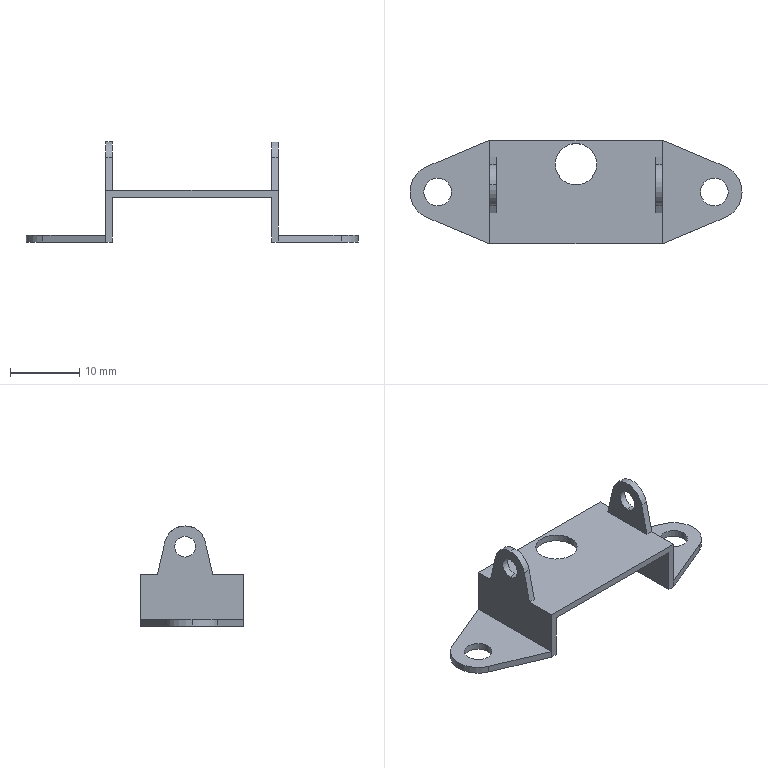Part | SolidWorks | features ICE 4, Cut 1, Extrusion 1 | 2 solids | 40 faces | box 48 x 15 x 14.485 mm | volume 815.815 mm3 | plane 24 | cylinder 16 | commonest cylinder face diameters 6 x5 3 x4 4 x4 8 x3
STEP:
#1=CARTESIAN_POINT('',(-143.531,150.119,1.));
#2=VERTEX_POINT('',#1);
#3=CARTESIAN_POINT('',(-139.531,150.119,1.));
#4=VERTEX_POINT('',#3);
#5=CARTESIAN_POINT('',(-141.531,150.119,1.));
#6=DIRECTION('',(0.,0.,1.));
#7=DIRECTION('',(-1.,0.,0.));
#8=AXIS2_PLACEMENT_3D('',#5,#6,#7);
#9=CIRCLE('',#8,2.);
#10=EDGE_CURVE('',#2,#4,#9,.T.);
#11=ORIENTED_EDGE('',*,*,#10,.T.);
#12=CARTESIAN_POINT('',(-139.531,150.119,0.));
#13=VERTEX_POINT('',#12);
#14=CARTESIAN_POINT('',(-139.531,150.119,1.));
#15=DIRECTION('',(0.,0.,-1.));
#16=VECTOR('',#15,1000.);
#17=LINE('',#14,#16);
#18=EDGE_CURVE('',#4,#13,#17,.T.);
#19=ORIENTED_EDGE('',*,*,#18,.T.);
#20=CARTESIAN_POINT('',(-143.531,150.119,0.));
#21=VERTEX_POINT('',#20);
#22=CARTESIAN_POINT('',(-141.531,150.119,0.));
#23=DIRECTION('',(0.,0.,1.));
#24=DIRECTION('',(-1.,0.,0.));
#25=AXIS2_PLACEMENT_3D('',#22,#23,#24);
#26=CIRCLE('',#25,2.);
#27=EDGE_CURVE('',#21,#13,#26,.T.);
#28=ORIENTED_EDGE('',*,*,#27,.F.);
#29=CARTESIAN_POINT('',(-143.531,150.119,1.));
#30=DIRECTION('',(0.,0.,-1.));
#31=VECTOR('',#30,1000.);
#32=LINE('',#29,#31);
#33=EDGE_CURVE('',#2,#21,#32,.T.);
#34=ORIENTED_EDGE('',*,*,#33,.F.);
#35=EDGE_LOOP('',(#11,#19,#28,#34));
#36=FACE_OUTER_BOUND('',#35,.T.);
#37=CARTESIAN_POINT('',(-141.531,150.119,1.));
#38=DIRECTION('',(0.,0.,-1.));
#39=DIRECTION('',(-1.,0.,0.));
#40=AXIS2_PLACEMENT_3D('',#37,#38,#39);
#41=CYLINDRICAL_SURFACE('',#40,2.);
#42=ADVANCED_FACE('',(#36),#41,.F.);
#43=CARTESIAN_POINT('',(-145.531,150.119,1.));
#44=VERTEX_POINT('',#43);
#45=CARTESIAN_POINT('',(-143.084,146.433,1.));
#46=VERTEX_POINT('',#45);
#47=CARTESIAN_POINT('',(-141.531,150.119,1.));
#48=DIRECTION('',(0.,0.,1.));
#49=DIRECTION('',(-1.,0.,0.));
#50=AXIS2_PLACEMENT_3D('',#47,#48,#49);
#51=CIRCLE('',#50,4.);
#52=EDGE_CURVE('',#44,#46,#51,.T.);
#53=ORIENTED_EDGE('',*,*,#52,.F.);
#54=CARTESIAN_POINT('',(-145.531,150.119,0.));
#55=VERTEX_POINT('',#54);
#56=CARTESIAN_POINT('',(-145.531,150.119,1.));
#57=DIRECTION('',(0.,0.,-1.));
#58=VECTOR('',#57,1000.);
#59=LINE('',#56,#58);
#60=EDGE_CURVE('',#44,#55,#59,.T.);
#61=ORIENTED_EDGE('',*,*,#60,.T.);
#62=CARTESIAN_POINT('',(-143.084,146.433,0.));
#63=VERTEX_POINT('',#62);
#64=CARTESIAN_POINT('',(-141.531,150.119,0.));
#65=DIRECTION('',(0.,0.,1.));
#66=DIRECTION('',(-1.,0.,0.));
#67=AXIS2_PLACEMENT_3D('',#64,#65,#66);
#68=CIRCLE('',#67,4.);
#69=EDGE_CURVE('',#55,#63,#68,.T.);
#70=ORIENTED_EDGE('',*,*,#69,.T.);
#71=CARTESIAN_POINT('',(-143.084,146.433,1.));
#72=DIRECTION('',(0.,0.,-1.));
#73=VECTOR('',#72,1000.);
#74=LINE('',#71,#73);
#75=EDGE_CURVE('',#46,#63,#74,.T.);
#76=ORIENTED_EDGE('',*,*,#75,.F.);
#77=EDGE_LOOP('',(#53,#61,#70,#76));
#78=FACE_OUTER_BOUND('',#77,.T.);
#79=CARTESIAN_POINT('',(-141.531,150.119,1.));
#80=DIRECTION('',(0.,0.,-1.));
#81=DIRECTION('',(-1.,0.,0.));
#82=AXIS2_PLACEMENT_3D('',#79,#80,#81);
#83=CYLINDRICAL_SURFACE('',#82,4.);
#84=ADVANCED_FACE('',(#78),#83,.T.);
#85=CARTESIAN_POINT('',(-143.084,153.805,1.));
#86=VERTEX_POINT('',#85);
#87=CARTESIAN_POINT('',(-141.531,150.119,1.));
#88=DIRECTION('',(0.,0.,1.));
#89=DIRECTION('',(-1.,0.,0.));
#90=AXIS2_PLACEMENT_3D('',#87,#88,#89);
#91=CIRCLE('',#90,4.);
#92=EDGE_CURVE('',#86,#44,#91,.T.);
#93=ORIENTED_EDGE('',*,*,#92,.T.);
#94=ORIENTED_EDGE('',*,*,#52,.T.);
#95=CARTESIAN_POINT('',(-134.031,142.619,1.));
#96=VERTEX_POINT('',#95);
#97=CARTESIAN_POINT('',(-143.084,146.433,1.));
#98=DIRECTION('',(0.9216,-0.3882,0.));
#99=VECTOR('',#98,1000.);
#100=LINE('',#97,#99);
#101=EDGE_CURVE('',#46,#96,#100,.T.);
#102=ORIENTED_EDGE('',*,*,#101,.T.);
#103=CARTESIAN_POINT('',(-134.031,157.619,1.));
#104=VERTEX_POINT('',#103);
#105=CARTESIAN_POINT('',(-134.031,157.619,1.));
#106=DIRECTION('',(0.,1.,0.));
#107=VECTOR('',#106,1000.);
#108=LINE('',#105,#107);
#109=EDGE_CURVE('',#96,#104,#108,.T.);
#110=ORIENTED_EDGE('',*,*,#109,.T.);
#111=CARTESIAN_POINT('',(-143.084,153.805,1.));
#112=DIRECTION('',(-0.9216,-0.3882,0.));
#113=VECTOR('',#112,1000.);
#114=LINE('',#111,#113);
#115=EDGE_CURVE('',#104,#86,#114,.T.);
#116=ORIENTED_EDGE('',*,*,#115,.T.);
#117=EDGE_LOOP('',(#93,#94,#102,#110,#116));
#118=FACE_OUTER_BOUND('',#117,.T.);
#119=ORIENTED_EDGE('',*,*,#10,.F.);
#120=CARTESIAN_POINT('',(-141.531,150.119,1.));
#121=DIRECTION('',(0.,0.,1.));
#122=DIRECTION('',(-1.,0.,0.));
#123=AXIS2_PLACEMENT_3D('',#120,#121,#122);
#124=CIRCLE('',#123,2.);
#125=EDGE_CURVE('',#4,#2,#124,.T.);
#126=ORIENTED_EDGE('',*,*,#125,.F.);
#127=EDGE_LOOP('',(#119,#126));
#128=FACE_BOUND('',#127,.T.);
#129=CARTESIAN_POINT('',(-141.531,150.119,1.));
#130=DIRECTION('',(0.,0.,-1.));
#131=DIRECTION('',(-1.,0.,0.));
#132=AXIS2_PLACEMENT_3D('',#129,#130,#131);
#133=PLANE('',#132);
#134=ADVANCED_FACE('',(#118,#128),#133,.F.);
#135=CARTESIAN_POINT('',(-143.084,153.805,0.));
#136=VERTEX_POINT('',#135);
#137=CARTESIAN_POINT('',(-141.531,150.119,0.));
#138=DIRECTION('',(0.,0.,1.));
#139=DIRECTION('',(-1.,0.,0.));
#140=AXIS2_PLACEMENT_3D('',#137,#138,#139);
#141=CIRCLE('',#140,4.);
#142=EDGE_CURVE('',#136,#55,#141,.T.);
#143=ORIENTED_EDGE('',*,*,#142,.F.);
#144=CARTESIAN_POINT('',(-134.031,157.619,0.));
#145=VERTEX_POINT('',#144);
#146=CARTESIAN_POINT('',(-143.084,153.805,0.));
#147=DIRECTION('',(-0.9216,-0.3882,0.));
#148=VECTOR('',#147,1000.);
#149=LINE('',#146,#148);
#150=EDGE_CURVE('',#145,#136,#149,.T.);
#151=ORIENTED_EDGE('',*,*,#150,.F.);
#152=CARTESIAN_POINT('',(-134.031,142.619,0.));
#153=VERTEX_POINT('',#152);
#154=CARTESIAN_POINT('',(-134.031,157.619,0.));
#155=DIRECTION('',(0.,1.,0.));
#156=VECTOR('',#155,1000.);
#157=LINE('',#154,#156);
#158=EDGE_CURVE('',#153,#145,#157,.T.);
#159=ORIENTED_EDGE('',*,*,#158,.F.);
#160=CARTESIAN_POINT('',(-143.084,146.433,0.));
#161=DIRECTION('',(0.9216,-0.3882,0.));
#162=VECTOR('',#161,1000.);
#163=LINE('',#160,#162);
#164=EDGE_CURVE('',#63,#153,#163,.T.);
#165=ORIENTED_EDGE('',*,*,#164,.F.);
#166=ORIENTED_EDGE('',*,*,#69,.F.);
#167=EDGE_LOOP('',(#143,#151,#159,#165,#166));
#168=FACE_OUTER_BOUND('',#167,.T.);
#169=ORIENTED_EDGE('',*,*,#27,.T.);
#170=CARTESIAN_POINT('',(-141.531,150.119,0.));
#171=DIRECTION('',(0.,0.,1.));
#172=DIRECTION('',(-1.,0.,0.));
#173=AXIS2_PLACEMENT_3D('',#170,#171,#172);
#174=CIRCLE('',#173,2.);
#175=EDGE_CURVE('',#13,#21,#174,.T.);
#176=ORIENTED_EDGE('',*,*,#175,.T.);
#177=EDGE_LOOP('',(#169,#176));
#178=FACE_BOUND('',#177,.T.);
#179=CARTESIAN_POINT('',(-141.531,150.119,0.));
#180=DIRECTION('',(0.,0.,-1.));
#181=DIRECTION('',(-1.,0.,0.));
#182=AXIS2_PLACEMENT_3D('',#179,#180,#181);
#183=PLANE('',#182);
#184=ADVANCED_FACE('',(#168,#178),#183,.T.);
#185=ORIENTED_EDGE('',*,*,#60,.F.);
#186=ORIENTED_EDGE('',*,*,#92,.F.);
#187=CARTESIAN_POINT('',(-143.084,153.805,1.));
#188=DIRECTION('',(0.,0.,-1.));
#189=VECTOR('',#188,1000.);
#190=LINE('',#187,#189);
#191=EDGE_CURVE('',#86,#136,#190,.T.);
#192=ORIENTED_EDGE('',*,*,#191,.T.);
#193=ORIENTED_EDGE('',*,*,#142,.T.);
#194=EDGE_LOOP('',(#185,#186,#192,#193));
#195=FACE_OUTER_BOUND('',#194,.T.);
#196=CARTESIAN_POINT('',(-141.531,150.119,1.));
#197=DIRECTION('',(0.,0.,-1.));
#198=DIRECTION('',(-1.,0.,0.));
#199=AXIS2_PLACEMENT_3D('',#196,#197,#198);
#200=CYLINDRICAL_SURFACE('',#199,4.);
#201=ADVANCED_FACE('',(#195),#200,.T.);
#202=ORIENTED_EDGE('',*,*,#164,.T.);
#203=CARTESIAN_POINT('',(-134.031,142.619,1.));
#204=DIRECTION('',(0.,0.,-1.));
#205=VECTOR('',#204,1000.);
#206=LINE('',#203,#205);
#207=EDGE_CURVE('',#96,#153,#206,.T.);
#208=ORIENTED_EDGE('',*,*,#207,.F.);
#209=ORIENTED_EDGE('',*,*,#101,.F.);
#210=ORIENTED_EDGE('',*,*,#75,.T.);
#211=EDGE_LOOP('',(#202,#208,#209,#210));
#212=FACE_OUTER_BOUND('',#211,.T.);
#213=CARTESIAN_POINT('',(-143.084,146.433,1.));
#214=DIRECTION('',(0.3882,0.9216,0.));
#215=DIRECTION('',(-0.9216,0.3882,0.));
#216=AXIS2_PLACEMENT_3D('',#213,#214,#215);
#217=PLANE('',#216);
#218=ADVANCED_FACE('',(#212),#217,.F.);
#219=ORIENTED_EDGE('',*,*,#158,.T.);
#220=CARTESIAN_POINT('',(-134.031,157.619,1.));
#221=DIRECTION('',(0.,0.,-1.));
#222=VECTOR('',#221,1000.);
#223=LINE('',#220,#222);
#224=EDGE_CURVE('',#104,#145,#223,.T.);
#225=ORIENTED_EDGE('',*,*,#224,.F.);
#226=ORIENTED_EDGE('',*,*,#109,.F.);
#227=ORIENTED_EDGE('',*,*,#207,.T.);
#228=EDGE_LOOP('',(#219,#225,#226,#227));
#229=FACE_OUTER_BOUND('',#228,.T.);
#230=CARTESIAN_POINT('',(-134.031,157.619,1.));
#231=DIRECTION('',(-1.,0.,0.));
#232=DIRECTION('',(0.,0.,1.));
#233=AXIS2_PLACEMENT_3D('',#230,#231,#232);
#234=PLANE('',#233);
#235=ADVANCED_FACE('',(#229),#234,.F.);
#236=ORIENTED_EDGE('',*,*,#150,.T.);
#237=ORIENTED_EDGE('',*,*,#191,.F.);
#238=ORIENTED_EDGE('',*,*,#115,.F.);
#239=ORIENTED_EDGE('',*,*,#224,.T.);
#240=EDGE_LOOP('',(#236,#237,#238,#239));
#241=FACE_OUTER_BOUND('',#240,.T.);
#242=CARTESIAN_POINT('',(-143.084,153.805,1.));
#243=DIRECTION('',(0.3882,-0.9216,0.));
#244=DIRECTION('',(0.9216,0.3882,0.));
#245=AXIS2_PLACEMENT_3D('',#242,#243,#244);
#246=PLANE('',#245);
#247=ADVANCED_FACE('',(#241),#246,.F.);
#248=ORIENTED_EDGE('',*,*,#18,.F.);
#249=ORIENTED_EDGE('',*,*,#125,.T.);
#250=ORIENTED_EDGE('',*,*,#33,.T.);
#251=ORIENTED_EDGE('',*,*,#175,.F.);
#252=EDGE_LOOP('',(#248,#249,#250,#251));
#253=FACE_OUTER_BOUND('',#252,.T.);
#254=CARTESIAN_POINT('',(-141.531,150.119,1.));
#255=DIRECTION('',(0.,0.,-1.));
#256=DIRECTION('',(-1.,0.,0.));
#257=AXIS2_PLACEMENT_3D('',#254,#255,#256);
#258=CYLINDRICAL_SURFACE('',#257,2.);
#259=ADVANCED_FACE('',(#253),#258,.F.);
#260=CLOSED_SHELL('',(#42,#84,#134,#184,#201,#218,#235,#247,#259));
#261=MANIFOLD_SOLID_BREP('',#260);
#262=CARTESIAN_POINT('',(-110.031,151.119,12.985));
#263=VERTEX_POINT('',#262);
#264=CARTESIAN_POINT('',(-110.031,151.119,9.985));
#265=VERTEX_POINT('',#264);
#266=CARTESIAN_POINT('',(-110.031,151.119,11.485));
#267=DIRECTION('',(1.,0.,0.));
#268=DIRECTION('',(0.,0.,-1.));
#269=AXIS2_PLACEMENT_3D('',#266,#267,#268);
#270=CIRCLE('',#269,1.5);
#271=EDGE_CURVE('',#263,#265,#270,.T.);
#272=ORIENTED_EDGE('',*,*,#271,.F.);
#273=CARTESIAN_POINT('',(-109.031,151.119,12.985));
#274=VERTEX_POINT('',#273);
#275=CARTESIAN_POINT('',(-110.031,151.119,12.985));
#276=DIRECTION('',(1.,0.,0.));
#277=VECTOR('',#276,1000.);
#278=LINE('',#275,#277);
#279=EDGE_CURVE('',#263,#274,#278,.T.);
#280=ORIENTED_EDGE('',*,*,#279,.T.);
#281=CARTESIAN_POINT('',(-109.031,151.119,9.985));
#282=VERTEX_POINT('',#281);
#283=CARTESIAN_POINT('',(-109.031,151.119,11.485));
#284=DIRECTION('',(1.,0.,0.));
#285=DIRECTION('',(0.,0.,-1.));
#286=AXIS2_PLACEMENT_3D('',#283,#284,#285);
#287=CIRCLE('',#286,1.5);
#288=EDGE_CURVE('',#274,#282,#287,.T.);
#289=ORIENTED_EDGE('',*,*,#288,.T.);
#290=CARTESIAN_POINT('',(-110.031,151.119,9.985));
#291=DIRECTION('',(1.,0.,0.));
#292=VECTOR('',#291,1000.);
#293=LINE('',#290,#292);
#294=EDGE_CURVE('',#265,#282,#293,.T.);
#295=ORIENTED_EDGE('',*,*,#294,.F.);
#296=EDGE_LOOP('',(#272,#280,#289,#295));
#297=FACE_OUTER_BOUND('',#296,.T.);
#298=CARTESIAN_POINT('',(-110.031,151.119,11.485));
#299=DIRECTION('',(1.,0.,0.));
#300=DIRECTION('',(0.,0.,-1.));
#301=AXIS2_PLACEMENT_3D('',#298,#299,#300);
#302=CYLINDRICAL_SURFACE('',#301,1.5);
#303=ADVANCED_FACE('',(#297),#302,.F.);
#304=CARTESIAN_POINT('',(-133.031,151.119,14.485));
#305=VERTEX_POINT('',#304);
#306=CARTESIAN_POINT('',(-133.031,148.196,12.16));
#307=VERTEX_POINT('',#306);
#308=CARTESIAN_POINT('',(-133.031,151.119,11.485));
#309=DIRECTION('',(1.,0.,0.));
#310=DIRECTION('',(0.,0.,1.));
#311=AXIS2_PLACEMENT_3D('',#308,#309,#310);
#312=CIRCLE('',#311,3.);
#313=EDGE_CURVE('',#305,#307,#312,.T.);
#314=ORIENTED_EDGE('',*,*,#313,.F.);
#315=CARTESIAN_POINT('',(-134.031,151.119,14.485));
#316=VERTEX_POINT('',#315);
#317=CARTESIAN_POINT('',(-133.031,151.119,14.485));
#318=DIRECTION('',(-1.,0.,0.));
#319=VECTOR('',#318,1000.);
#320=LINE('',#317,#319);
#321=EDGE_CURVE('',#305,#316,#320,.T.);
#322=ORIENTED_EDGE('',*,*,#321,.T.);
#323=CARTESIAN_POINT('',(-134.031,148.196,12.16));
#324=VERTEX_POINT('',#323);
#325=CARTESIAN_POINT('',(-134.031,151.119,11.485));
#326=DIRECTION('',(1.,0.,0.));
#327=DIRECTION('',(0.,0.,1.));
#328=AXIS2_PLACEMENT_3D('',#325,#326,#327);
#329=CIRCLE('',#328,3.);
#330=EDGE_CURVE('',#316,#324,#329,.T.);
#331=ORIENTED_EDGE('',*,*,#330,.T.);
#332=CARTESIAN_POINT('',(-133.031,148.196,12.16));
#333=DIRECTION('',(-1.,0.,0.));
#334=VECTOR('',#333,1000.);
#335=LINE('',#332,#334);
#336=EDGE_CURVE('',#307,#324,#335,.T.);
#337=ORIENTED_EDGE('',*,*,#336,.F.);
#338=EDGE_LOOP('',(#314,#322,#331,#337));
#339=FACE_OUTER_BOUND('',#338,.T.);
#340=CARTESIAN_POINT('',(-133.031,151.119,11.485));
#341=DIRECTION('',(-1.,0.,0.));
#342=DIRECTION('',(0.,0.,1.));
#343=AXIS2_PLACEMENT_3D('',#340,#341,#342);
#344=CYLINDRICAL_SURFACE('',#343,3.);
#345=ADVANCED_FACE('',(#339),#344,.T.);
#346=CARTESIAN_POINT('',(-133.031,151.119,9.985));
#347=VERTEX_POINT('',#346);
#348=CARTESIAN_POINT('',(-133.031,151.119,12.985));
#349=VERTEX_POINT('',#348);
#350=CARTESIAN_POINT('',(-133.031,151.119,11.485));
#351=DIRECTION('',(-1.,0.,0.));
#352=DIRECTION('',(0.,0.,1.));
#353=AXIS2_PLACEMENT_3D('',#350,#351,#352);
#354=CIRCLE('',#353,1.5);
#355=EDGE_CURVE('',#347,#349,#354,.T.);
#356=ORIENTED_EDGE('',*,*,#355,.F.);
#357=CARTESIAN_POINT('',(-134.031,151.119,9.985));
#358=VERTEX_POINT('',#357);
#359=CARTESIAN_POINT('',(-133.031,151.119,9.985));
#360=DIRECTION('',(-1.,0.,0.));
#361=VECTOR('',#360,1000.);
#362=LINE('',#359,#361);
#363=EDGE_CURVE('',#347,#358,#362,.T.);
#364=ORIENTED_EDGE('',*,*,#363,.T.);
#365=CARTESIAN_POINT('',(-134.031,151.119,12.985));
#366=VERTEX_POINT('',#365);
#367=CARTESIAN_POINT('',(-134.031,151.119,11.485));
#368=DIRECTION('',(-1.,0.,0.));
#369=DIRECTION('',(0.,0.,1.));
#370=AXIS2_PLACEMENT_3D('',#367,#368,#369);
#371=CIRCLE('',#370,1.5);
#372=EDGE_CURVE('',#358,#366,#371,.T.);
#373=ORIENTED_EDGE('',*,*,#372,.T.);
#374=CARTESIAN_POINT('',(-133.031,151.119,12.985));
#375=DIRECTION('',(-1.,0.,0.));
#376=VECTOR('',#375,1000.);
#377=LINE('',#374,#376);
#378=EDGE_CURVE('',#349,#366,#377,.T.);
#379=ORIENTED_EDGE('',*,*,#378,.F.);
#380=EDGE_LOOP('',(#356,#364,#373,#379));
#381=FACE_OUTER_BOUND('',#380,.T.);
#382=CARTESIAN_POINT('',(-133.031,151.119,11.485));
#383=DIRECTION('',(-1.,0.,0.));
#384=DIRECTION('',(0.,0.,1.));
#385=AXIS2_PLACEMENT_3D('',#382,#383,#384);
#386=CYLINDRICAL_SURFACE('',#385,1.5);
#387=ADVANCED_FACE('',(#381),#386,.F.);
#388=CARTESIAN_POINT('',(-124.531,154.119,7.5));
#389=VERTEX_POINT('',#388);
#390=CARTESIAN_POINT('',(-118.531,154.119,7.5));
#391=VERTEX_POINT('',#390);
#392=CARTESIAN_POINT('',(-121.531,154.119,7.5));
#393=DIRECTION('',(0.,0.,1.));
#394=DIRECTION('',(1.,0.,0.));
#395=AXIS2_PLACEMENT_3D('',#392,#393,#394);
#396=CIRCLE('',#395,3.);
#397=EDGE_CURVE('',#389,#391,#396,.T.);
#398=ORIENTED_EDGE('',*,*,#397,.T.);
#399=CARTESIAN_POINT('',(-118.531,154.119,6.5));
#400=VERTEX_POINT('',#399);
#401=CARTESIAN_POINT('',(-118.531,154.119,7.5));
#402=DIRECTION('',(0.,0.,-1.));
#403=VECTOR('',#402,1000.);
#404=LINE('',#401,#403);
#405=EDGE_CURVE('',#391,#400,#404,.T.);
#406=ORIENTED_EDGE('',*,*,#405,.T.);
#407=CARTESIAN_POINT('',(-124.531,154.119,6.5));
#408=VERTEX_POINT('',#407);
#409=CARTESIAN_POINT('',(-121.531,154.119,6.5));
#410=DIRECTION('',(0.,0.,1.));
#411=DIRECTION('',(1.,0.,0.));
#412=AXIS2_PLACEMENT_3D('',#409,#410,#411);
#413=CIRCLE('',#412,3.);
#414=EDGE_CURVE('',#408,#400,#413,.T.);
#415=ORIENTED_EDGE('',*,*,#414,.F.);
#416=CARTESIAN_POINT('',(-124.531,154.119,7.5));
#417=DIRECTION('',(0.,0.,-1.));
#418=VECTOR('',#417,1000.);
#419=LINE('',#416,#418);
#420=EDGE_CURVE('',#389,#408,#419,.T.);
#421=ORIENTED_EDGE('',*,*,#420,.F.);
#422=EDGE_LOOP('',(#398,#406,#415,#421));
#423=FACE_OUTER_BOUND('',#422,.T.);
#424=CARTESIAN_POINT('',(-121.531,154.119,7.5));
#425=DIRECTION('',(0.,0.,-1.));
#426=DIRECTION('',(-1.,0.,0.));
#427=AXIS2_PLACEMENT_3D('',#424,#425,#426);
#428=CYLINDRICAL_SURFACE('',#427,3.);
#429=ADVANCED_FACE('',(#423),#428,.F.);
#430=CARTESIAN_POINT('',(-103.531,150.119,1.));
#431=VERTEX_POINT('',#430);
#432=CARTESIAN_POINT('',(-99.531,150.119,1.));
#433=VERTEX_POINT('',#432);
#434=CARTESIAN_POINT('',(-101.531,150.119,1.));
#435=DIRECTION('',(0.,0.,1.));
#436=DIRECTION('',(1.,0.,0.));
#437=AXIS2_PLACEMENT_3D('',#434,#435,#436);
#438=CIRCLE('',#437,2.);
#439=EDGE_CURVE('',#431,#433,#438,.T.);
#440=ORIENTED_EDGE('',*,*,#439,.T.);
#441=CARTESIAN_POINT('',(-99.531,150.119,0.));
#442=VERTEX_POINT('',#441);
#443=CARTESIAN_POINT('',(-99.531,150.119,1.));
#444=DIRECTION('',(0.,0.,-1.));
#445=VECTOR('',#444,1000.);
#446=LINE('',#443,#445);
#447=EDGE_CURVE('',#433,#442,#446,.T.);
#448=ORIENTED_EDGE('',*,*,#447,.T.);
#449=CARTESIAN_POINT('',(-103.531,150.119,0.));
#450=VERTEX_POINT('',#449);
#451=CARTESIAN_POINT('',(-101.531,150.119,0.));
#452=DIRECTION('',(0.,0.,1.));
#453=DIRECTION('',(1.,0.,0.));
#454=AXIS2_PLACEMENT_3D('',#451,#452,#453);
#455=CIRCLE('',#454,2.);
#456=EDGE_CURVE('',#450,#442,#455,.T.);
#457=ORIENTED_EDGE('',*,*,#456,.F.);
#458=CARTESIAN_POINT('',(-103.531,150.119,1.));
#459=DIRECTION('',(0.,0.,-1.));
#460=VECTOR('',#459,1000.);
#461=LINE('',#458,#460);
#462=EDGE_CURVE('',#431,#450,#461,.T.);
#463=ORIENTED_EDGE('',*,*,#462,.F.);
#464=EDGE_LOOP('',(#440,#448,#457,#463));
#465=FACE_OUTER_BOUND('',#464,.T.);
#466=CARTESIAN_POINT('',(-101.531,150.119,1.));
#467=DIRECTION('',(0.,0.,-1.));
#468=DIRECTION('',(-1.,0.,0.));
#469=AXIS2_PLACEMENT_3D('',#466,#467,#468);
#470=CYLINDRICAL_SURFACE('',#469,2.);
#471=ADVANCED_FACE('',(#465),#470,.F.);
#472=ORIENTED_EDGE('',*,*,#414,.T.);
#473=CARTESIAN_POINT('',(-121.531,154.119,6.5));
#474=DIRECTION('',(0.,0.,1.));
#475=DIRECTION('',(1.,0.,0.));
#476=AXIS2_PLACEMENT_3D('',#473,#474,#475);
#477=CIRCLE('',#476,3.);
#478=EDGE_CURVE('',#400,#408,#477,.T.);
#479=ORIENTED_EDGE('',*,*,#478,.T.);
#480=EDGE_LOOP('',(#472,#479));
#481=FACE_BOUND('',#480,.T.);
#482=CARTESIAN_POINT('',(-133.031,142.619,6.5));
#483=VERTEX_POINT('',#482);
#484=CARTESIAN_POINT('',(-110.031,142.619,6.5));
#485=VERTEX_POINT('',#484);
#486=CARTESIAN_POINT('',(-109.031,142.619,6.5));
#487=DIRECTION('',(1.,0.,0.));
#488=VECTOR('',#487,1000.);
#489=LINE('',#486,#488);
#490=EDGE_CURVE('',#483,#485,#489,.T.);
#491=ORIENTED_EDGE('',*,*,#490,.F.);
#492=CARTESIAN_POINT('',(-133.031,157.619,6.5));
#493=VERTEX_POINT('',#492);
#494=CARTESIAN_POINT('',(-133.031,0.,6.5));
#495=DIRECTION('',(0.,1.,0.));
#496=VECTOR('',#495,1000.);
#497=LINE('',#494,#496);
#498=EDGE_CURVE('',#483,#493,#497,.T.);
#499=ORIENTED_EDGE('',*,*,#498,.T.);
#500=CARTESIAN_POINT('',(-110.031,157.619,6.5));
#501=VERTEX_POINT('',#500);
#502=CARTESIAN_POINT('',(-109.031,157.619,6.5));
#503=DIRECTION('',(-1.,0.,0.));
#504=VECTOR('',#503,1000.);
#505=LINE('',#502,#504);
#506=EDGE_CURVE('',#501,#493,#505,.T.);
#507=ORIENTED_EDGE('',*,*,#506,.F.);
#508=CARTESIAN_POINT('',(-110.031,157.619,6.5));
#509=DIRECTION('',(0.,-1.,0.));
#510=VECTOR('',#509,1000.);
#511=LINE('',#508,#510);
#512=EDGE_CURVE('',#501,#485,#511,.T.);
#513=ORIENTED_EDGE('',*,*,#512,.T.);
#514=EDGE_LOOP('',(#491,#499,#507,#513));
#515=FACE_OUTER_BOUND('',#514,.T.);
#516=CARTESIAN_POINT('',(0.,0.,6.5));
#517=DIRECTION('',(0.,0.,-1.));
#518=DIRECTION('',(-1.,0.,0.));
#519=AXIS2_PLACEMENT_3D('',#516,#517,#518);
#520=PLANE('',#519);
#521=ADVANCED_FACE('',(#481,#515),#520,.T.);
#522=CARTESIAN_POINT('',(-99.978,146.433,1.));
#523=VERTEX_POINT('',#522);
#524=CARTESIAN_POINT('',(-99.978,153.805,1.));
#525=VERTEX_POINT('',#524);
#526=CARTESIAN_POINT('',(-101.531,150.119,1.));
#527=DIRECTION('',(0.,0.,1.));
#528=DIRECTION('',(1.,0.,0.));
#529=AXIS2_PLACEMENT_3D('',#526,#527,#528);
#530=CIRCLE('',#529,4.);
#531=EDGE_CURVE('',#523,#525,#530,.T.);
#532=ORIENTED_EDGE('',*,*,#531,.T.);
#533=CARTESIAN_POINT('',(-109.031,157.619,1.));
#534=VERTEX_POINT('',#533);
#535=CARTESIAN_POINT('',(-99.978,153.805,1.));
#536=DIRECTION('',(-0.9216,0.3882,0.));
#537=VECTOR('',#536,1000.);
#538=LINE('',#535,#537);
#539=EDGE_CURVE('',#525,#534,#538,.T.);
#540=ORIENTED_EDGE('',*,*,#539,.T.);
#541=CARTESIAN_POINT('',(-109.031,142.619,1.));
#542=VERTEX_POINT('',#541);
#543=CARTESIAN_POINT('',(-109.031,157.619,1.));
#544=DIRECTION('',(0.,-1.,0.));
#545=VECTOR('',#544,1000.);
#546=LINE('',#543,#545);
#547=EDGE_CURVE('',#534,#542,#546,.T.);
#548=ORIENTED_EDGE('',*,*,#547,.T.);
#549=CARTESIAN_POINT('',(-99.978,146.433,1.));
#550=DIRECTION('',(0.9216,0.3882,0.));
#551=VECTOR('',#550,1000.);
#552=LINE('',#549,#551);
#553=EDGE_CURVE('',#542,#523,#552,.T.);
#554=ORIENTED_EDGE('',*,*,#553,.T.);
#555=EDGE_LOOP('',(#532,#540,#548,#554));
#556=FACE_OUTER_BOUND('',#555,.T.);
#557=ORIENTED_EDGE('',*,*,#439,.F.);
#558=CARTESIAN_POINT('',(-101.531,150.119,1.));
#559=DIRECTION('',(0.,0.,1.));
#560=DIRECTION('',(1.,0.,0.));
#561=AXIS2_PLACEMENT_3D('',#558,#559,#560);
#562=CIRCLE('',#561,2.);
#563=EDGE_CURVE('',#433,#431,#562,.T.);
#564=ORIENTED_EDGE('',*,*,#563,.F.);
#565=EDGE_LOOP('',(#557,#564));
#566=FACE_BOUND('',#565,.T.);
#567=CARTESIAN_POINT('',(-101.531,150.119,1.));
#568=DIRECTION('',(0.,0.,1.));
#569=DIRECTION('',(1.,0.,0.));
#570=AXIS2_PLACEMENT_3D('',#567,#568,#569);
#571=PLANE('',#570);
#572=ADVANCED_FACE('',(#556,#566),#571,.T.);
#573=CARTESIAN_POINT('',(-99.978,146.433,0.));
#574=VERTEX_POINT('',#573);
#575=CARTESIAN_POINT('',(-99.978,153.805,0.));
#576=VERTEX_POINT('',#575);
#577=CARTESIAN_POINT('',(-101.531,150.119,0.));
#578=DIRECTION('',(0.,0.,1.));
#579=DIRECTION('',(1.,0.,0.));
#580=AXIS2_PLACEMENT_3D('',#577,#578,#579);
#581=CIRCLE('',#580,4.);
#582=EDGE_CURVE('',#574,#576,#581,.T.);
#583=ORIENTED_EDGE('',*,*,#582,.F.);
#584=CARTESIAN_POINT('',(-109.031,142.619,0.));
#585=VERTEX_POINT('',#584);
#586=CARTESIAN_POINT('',(-99.978,146.433,0.));
#587=DIRECTION('',(0.9216,0.3882,0.));
#588=VECTOR('',#587,1000.);
#589=LINE('',#586,#588);
#590=EDGE_CURVE('',#585,#574,#589,.T.);
#591=ORIENTED_EDGE('',*,*,#590,.F.);
#592=CARTESIAN_POINT('',(-110.031,142.619,0.));
#593=VERTEX_POINT('',#592);
#594=CARTESIAN_POINT('',(-110.031,142.619,0.));
#595=DIRECTION('',(1.,0.,0.));
#596=VECTOR('',#595,1000.);
#597=LINE('',#594,#596);
#598=EDGE_CURVE('',#593,#585,#597,.T.);
#599=ORIENTED_EDGE('',*,*,#598,.F.);
#600=CARTESIAN_POINT('',(-110.031,157.619,0.));
#601=VERTEX_POINT('',#600);
#602=CARTESIAN_POINT('',(-110.031,157.619,0.));
#603=DIRECTION('',(0.,-1.,0.));
#604=VECTOR('',#603,1000.);
#605=LINE('',#602,#604);
#606=EDGE_CURVE('',#601,#593,#605,.T.);
#607=ORIENTED_EDGE('',*,*,#606,.F.);
#608=CARTESIAN_POINT('',(-109.031,157.619,0.));
#609=VERTEX_POINT('',#608);
#610=CARTESIAN_POINT('',(-110.031,157.619,0.));
#611=DIRECTION('',(-1.,0.,0.));
#612=VECTOR('',#611,1000.);
#613=LINE('',#610,#612);
#614=EDGE_CURVE('',#609,#601,#613,.T.);
#615=ORIENTED_EDGE('',*,*,#614,.F.);
#616=CARTESIAN_POINT('',(-99.978,153.805,0.));
#617=DIRECTION('',(-0.9216,0.3882,0.));
#618=VECTOR('',#617,1000.);
#619=LINE('',#616,#618);
#620=EDGE_CURVE('',#576,#609,#619,.T.);
#621=ORIENTED_EDGE('',*,*,#620,.F.);
#622=EDGE_LOOP('',(#583,#591,#599,#607,#615,#621));
#623=FACE_OUTER_BOUND('',#622,.T.);
#624=ORIENTED_EDGE('',*,*,#456,.T.);
#625=CARTESIAN_POINT('',(-101.531,150.119,0.));
#626=DIRECTION('',(0.,0.,1.));
#627=DIRECTION('',(1.,0.,0.));
#628=AXIS2_PLACEMENT_3D('',#625,#626,#627);
#629=CIRCLE('',#628,2.);
#630=EDGE_CURVE('',#442,#450,#629,.T.);
#631=ORIENTED_EDGE('',*,*,#630,.T.);
#632=EDGE_LOOP('',(#624,#631));
#633=FACE_BOUND('',#632,.T.);
#634=CARTESIAN_POINT('',(-101.531,150.119,0.));
#635=DIRECTION('',(0.,0.,1.));
#636=DIRECTION('',(1.,0.,0.));
#637=AXIS2_PLACEMENT_3D('',#634,#635,#636);
#638=PLANE('',#637);
#639=ADVANCED_FACE('',(#623,#633),#638,.F.);
#640=ORIENTED_EDGE('',*,*,#582,.T.);
#641=CARTESIAN_POINT('',(-99.978,153.805,1.));
#642=DIRECTION('',(0.,0.,-1.));
#643=VECTOR('',#642,1000.);
#644=LINE('',#641,#643);
#645=EDGE_CURVE('',#525,#576,#644,.T.);
#646=ORIENTED_EDGE('',*,*,#645,.F.);
#647=ORIENTED_EDGE('',*,*,#531,.F.);
#648=CARTESIAN_POINT('',(-99.978,146.433,1.));
#649=DIRECTION('',(0.,0.,-1.));
#650=VECTOR('',#649,1000.);
#651=LINE('',#648,#650);
#652=EDGE_CURVE('',#523,#574,#651,.T.);
#653=ORIENTED_EDGE('',*,*,#652,.T.);
#654=EDGE_LOOP('',(#640,#646,#647,#653));
#655=FACE_OUTER_BOUND('',#654,.T.);
#656=CARTESIAN_POINT('',(-101.531,150.119,1.));
#657=DIRECTION('',(0.,0.,-1.));
#658=DIRECTION('',(-1.,0.,0.));
#659=AXIS2_PLACEMENT_3D('',#656,#657,#658);
#660=CYLINDRICAL_SURFACE('',#659,4.);
#661=ADVANCED_FACE('',(#655),#660,.T.);
#662=ORIENTED_EDGE('',*,*,#620,.T.);
#663=CARTESIAN_POINT('',(-109.031,157.619,1.));
#664=DIRECTION('',(0.,0.,-1.));
#665=VECTOR('',#664,1000.);
#666=LINE('',#663,#665);
#667=EDGE_CURVE('',#534,#609,#666,.T.);
#668=ORIENTED_EDGE('',*,*,#667,.F.);
#669=ORIENTED_EDGE('',*,*,#539,.F.);
#670=ORIENTED_EDGE('',*,*,#645,.T.);
#671=EDGE_LOOP('',(#662,#668,#669,#670));
#672=FACE_OUTER_BOUND('',#671,.T.);
#673=CARTESIAN_POINT('',(-99.978,153.805,1.));
#674=DIRECTION('',(-0.3882,-0.9216,0.));
#675=DIRECTION('',(0.9216,-0.3882,0.));
#676=AXIS2_PLACEMENT_3D('',#673,#674,#675);
#677=PLANE('',#676);
#678=ADVANCED_FACE('',(#672),#677,.F.);
#679=ORIENTED_EDGE('',*,*,#590,.T.);
#680=ORIENTED_EDGE('',*,*,#652,.F.);
#681=ORIENTED_EDGE('',*,*,#553,.F.);
#682=CARTESIAN_POINT('',(-109.031,142.619,1.));
#683=DIRECTION('',(0.,0.,-1.));
#684=VECTOR('',#683,1000.);
#685=LINE('',#682,#684);
#686=EDGE_CURVE('',#542,#585,#685,.T.);
#687=ORIENTED_EDGE('',*,*,#686,.T.);
#688=EDGE_LOOP('',(#679,#680,#681,#687));
#689=FACE_OUTER_BOUND('',#688,.T.);
#690=CARTESIAN_POINT('',(-99.978,146.433,1.));
#691=DIRECTION('',(-0.3882,0.9216,0.));
#692=DIRECTION('',(-0.9216,-0.3882,0.));
#693=AXIS2_PLACEMENT_3D('',#690,#691,#692);
#694=PLANE('',#693);
#695=ADVANCED_FACE('',(#689),#694,.F.);
#696=ORIENTED_EDGE('',*,*,#447,.F.);
#697=ORIENTED_EDGE('',*,*,#563,.T.);
#698=ORIENTED_EDGE('',*,*,#462,.T.);
#699=ORIENTED_EDGE('',*,*,#630,.F.);
#700=EDGE_LOOP('',(#696,#697,#698,#699));
#701=FACE_OUTER_BOUND('',#700,.T.);
#702=CARTESIAN_POINT('',(-101.531,150.119,1.));
#703=DIRECTION('',(0.,0.,-1.));
#704=DIRECTION('',(-1.,0.,0.));
#705=AXIS2_PLACEMENT_3D('',#702,#703,#704);
#706=CYLINDRICAL_SURFACE('',#705,2.);
#707=ADVANCED_FACE('',(#701),#706,.F.);
#708=ORIENTED_EDGE('',*,*,#606,.T.);
#709=CARTESIAN_POINT('',(-110.031,142.619,6.5));
#710=DIRECTION('',(0.,0.,-1.));
#711=VECTOR('',#710,1000.);
#712=LINE('',#709,#711);
#713=EDGE_CURVE('',#485,#593,#712,.T.);
#714=ORIENTED_EDGE('',*,*,#713,.F.);
#715=ORIENTED_EDGE('',*,*,#512,.F.);
#716=CARTESIAN_POINT('',(-110.031,157.619,6.5));
#717=DIRECTION('',(0.,0.,-1.));
#718=VECTOR('',#717,1000.);
#719=LINE('',#716,#718);
#720=EDGE_CURVE('',#501,#601,#719,.T.);
#721=ORIENTED_EDGE('',*,*,#720,.T.);
#722=EDGE_LOOP('',(#708,#714,#715,#721));
#723=FACE_OUTER_BOUND('',#722,.T.);
#724=CARTESIAN_POINT('',(-110.031,157.619,6.5));
#725=DIRECTION('',(1.,0.,0.));
#726=DIRECTION('',(0.,0.,-1.));
#727=AXIS2_PLACEMENT_3D('',#724,#725,#726);
#728=PLANE('',#727);
#729=ADVANCED_FACE('',(#723),#728,.F.);
#730=ORIENTED_EDGE('',*,*,#598,.T.);
#731=ORIENTED_EDGE('',*,*,#686,.F.);
#732=CARTESIAN_POINT('',(-109.031,142.619,7.5));
#733=VERTEX_POINT('',#732);
#734=CARTESIAN_POINT('',(-109.031,142.619,6.5));
#735=DIRECTION('',(0.,0.,-1.));
#736=VECTOR('',#735,1000.);
#737=LINE('',#734,#736);
#738=EDGE_CURVE('',#733,#542,#737,.T.);
#739=ORIENTED_EDGE('',*,*,#738,.F.);
#740=CARTESIAN_POINT('',(-134.031,142.619,7.5));
#741=VERTEX_POINT('',#740);
#742=CARTESIAN_POINT('',(-109.031,142.619,7.5));
#743=DIRECTION('',(1.,0.,0.));
#744=VECTOR('',#743,1000.);
#745=LINE('',#742,#744);
#746=EDGE_CURVE('',#741,#733,#745,.T.);
#747=ORIENTED_EDGE('',*,*,#746,.F.);
#748=CARTESIAN_POINT('',(-134.031,142.619,0.));
#749=VERTEX_POINT('',#748);
#750=CARTESIAN_POINT('',(-134.031,142.619,7.5));
#751=DIRECTION('',(0.,0.,-1.));
#752=VECTOR('',#751,1000.);
#753=LINE('',#750,#752);
#754=EDGE_CURVE('',#741,#749,#753,.T.);
#755=ORIENTED_EDGE('',*,*,#754,.T.);
#756=CARTESIAN_POINT('',(-133.031,142.619,0.));
#757=VERTEX_POINT('',#756);
#758=CARTESIAN_POINT('',(-133.031,142.619,0.));
#759=DIRECTION('',(1.,0.,0.));
#760=VECTOR('',#759,1000.);
#761=LINE('',#758,#760);
#762=EDGE_CURVE('',#749,#757,#761,.T.);
#763=ORIENTED_EDGE('',*,*,#762,.T.);
#764=CARTESIAN_POINT('',(-133.031,142.619,6.5));
#765=DIRECTION('',(0.,0.,-1.));
#766=VECTOR('',#765,1000.);
#767=LINE('',#764,#766);
#768=EDGE_CURVE('',#483,#757,#767,.T.);
#769=ORIENTED_EDGE('',*,*,#768,.F.);
#770=ORIENTED_EDGE('',*,*,#490,.T.);
#771=ORIENTED_EDGE('',*,*,#713,.T.);
#772=EDGE_LOOP('',(#730,#731,#739,#747,#755,#763,#769,#770,#771));
#773=FACE_OUTER_BOUND('',#772,.T.);
#774=CARTESIAN_POINT('',(-110.031,142.619,6.5));
#775=DIRECTION('',(0.,1.,0.));
#776=DIRECTION('',(0.,0.,1.));
#777=AXIS2_PLACEMENT_3D('',#774,#775,#776);
#778=PLANE('',#777);
#779=ADVANCED_FACE('',(#773),#778,.F.);
#780=ORIENTED_EDGE('',*,*,#547,.F.);
#781=CARTESIAN_POINT('',(-109.031,157.619,7.5));
#782=VERTEX_POINT('',#781);
#783=CARTESIAN_POINT('',(-109.031,157.619,6.5));
#784=DIRECTION('',(0.,0.,-1.));
#785=VECTOR('',#784,1000.);
#786=LINE('',#783,#785);
#787=EDGE_CURVE('',#782,#534,#786,.T.);
#788=ORIENTED_EDGE('',*,*,#787,.F.);
#789=CARTESIAN_POINT('',(-109.031,155.119,7.5));
#790=VERTEX_POINT('',#789);
#791=CARTESIAN_POINT('',(-109.031,157.619,7.5));
#792=DIRECTION('',(0.,1.,0.));
#793=VECTOR('',#792,1000.);
#794=LINE('',#791,#793);
#795=EDGE_CURVE('',#790,#782,#794,.T.);
#796=ORIENTED_EDGE('',*,*,#795,.F.);
#797=CARTESIAN_POINT('',(-109.031,154.042,12.16));
#798=VERTEX_POINT('',#797);
#799=CARTESIAN_POINT('',(-109.031,155.119,7.5));
#800=DIRECTION('',(0.,-0.2252,0.9743));
#801=VECTOR('',#800,1000.);
#802=LINE('',#799,#801);
#803=EDGE_CURVE('',#790,#798,#802,.T.);
#804=ORIENTED_EDGE('',*,*,#803,.T.);
#805=CARTESIAN_POINT('',(-109.031,148.196,12.16));
#806=VERTEX_POINT('',#805);
#807=CARTESIAN_POINT('',(-109.031,151.119,11.485));
#808=DIRECTION('',(1.,0.,0.));
#809=DIRECTION('',(0.,0.,-1.));
#810=AXIS2_PLACEMENT_3D('',#807,#808,#809);
#811=CIRCLE('',#810,3.);
#812=EDGE_CURVE('',#798,#806,#811,.T.);
#813=ORIENTED_EDGE('',*,*,#812,.T.);
#814=CARTESIAN_POINT('',(-109.031,147.119,7.5));
#815=VERTEX_POINT('',#814);
#816=CARTESIAN_POINT('',(-109.031,148.196,12.16));
#817=DIRECTION('',(0.,-0.2252,-0.9743));
#818=VECTOR('',#817,1000.);
#819=LINE('',#816,#818);
#820=EDGE_CURVE('',#806,#815,#819,.T.);
#821=ORIENTED_EDGE('',*,*,#820,.T.);
#822=CARTESIAN_POINT('',(-109.031,157.619,7.5));
#823=DIRECTION('',(0.,1.,0.));
#824=VECTOR('',#823,1000.);
#825=LINE('',#822,#824);
#826=EDGE_CURVE('',#733,#815,#825,.T.);
#827=ORIENTED_EDGE('',*,*,#826,.F.);
#828=ORIENTED_EDGE('',*,*,#738,.T.);
#829=EDGE_LOOP('',(#780,#788,#796,#804,#813,#821,#827,#828));
#830=FACE_OUTER_BOUND('',#829,.T.);
#831=CARTESIAN_POINT('',(-109.031,151.119,11.485));
#832=DIRECTION('',(1.,0.,0.));
#833=DIRECTION('',(0.,0.,-1.));
#834=AXIS2_PLACEMENT_3D('',#831,#832,#833);
#835=CIRCLE('',#834,1.5);
#836=EDGE_CURVE('',#282,#274,#835,.T.);
#837=ORIENTED_EDGE('',*,*,#836,.F.);
#838=ORIENTED_EDGE('',*,*,#288,.F.);
#839=EDGE_LOOP('',(#837,#838));
#840=FACE_BOUND('',#839,.T.);
#841=CARTESIAN_POINT('',(-109.031,157.619,6.5));
#842=DIRECTION('',(-1.,0.,0.));
#843=DIRECTION('',(0.,0.,1.));
#844=AXIS2_PLACEMENT_3D('',#841,#842,#843);
#845=PLANE('',#844);
#846=ADVANCED_FACE('',(#830,#840),#845,.F.);
#847=ORIENTED_EDGE('',*,*,#614,.T.);
#848=ORIENTED_EDGE('',*,*,#720,.F.);
#849=ORIENTED_EDGE('',*,*,#506,.T.);
#850=CARTESIAN_POINT('',(-133.031,157.619,0.));
#851=VERTEX_POINT('',#850);
#852=CARTESIAN_POINT('',(-133.031,157.619,6.5));
#853=DIRECTION('',(0.,0.,-1.));
#854=VECTOR('',#853,1000.);
#855=LINE('',#852,#854);
#856=EDGE_CURVE('',#493,#851,#855,.T.);
#857=ORIENTED_EDGE('',*,*,#856,.T.);
#858=CARTESIAN_POINT('',(-134.031,157.619,0.));
#859=VERTEX_POINT('',#858);
#860=CARTESIAN_POINT('',(-133.031,157.619,0.));
#861=DIRECTION('',(-1.,0.,0.));
#862=VECTOR('',#861,1000.);
#863=LINE('',#860,#862);
#864=EDGE_CURVE('',#851,#859,#863,.T.);
#865=ORIENTED_EDGE('',*,*,#864,.T.);
#866=CARTESIAN_POINT('',(-134.031,157.619,7.5));
#867=VERTEX_POINT('',#866);
#868=CARTESIAN_POINT('',(-134.031,157.619,7.5));
#869=DIRECTION('',(0.,0.,-1.));
#870=VECTOR('',#869,1000.);
#871=LINE('',#868,#870);
#872=EDGE_CURVE('',#867,#859,#871,.T.);
#873=ORIENTED_EDGE('',*,*,#872,.F.);
#874=CARTESIAN_POINT('',(-109.031,157.619,7.5));
#875=DIRECTION('',(-1.,0.,0.));
#876=VECTOR('',#875,1000.);
#877=LINE('',#874,#876);
#878=EDGE_CURVE('',#782,#867,#877,.T.);
#879=ORIENTED_EDGE('',*,*,#878,.F.);
#880=ORIENTED_EDGE('',*,*,#787,.T.);
#881=ORIENTED_EDGE('',*,*,#667,.T.);
#882=EDGE_LOOP('',(#847,#848,#849,#857,#865,#873,#879,#880,#881));
#883=FACE_OUTER_BOUND('',#882,.T.);
#884=CARTESIAN_POINT('',(-110.031,157.619,6.5));
#885=DIRECTION('',(0.,-1.,0.));
#886=DIRECTION('',(0.,0.,-1.));
#887=AXIS2_PLACEMENT_3D('',#884,#885,#886);
#888=PLANE('',#887);
#889=ADVANCED_FACE('',(#883),#888,.F.);
#890=CARTESIAN_POINT('',(-110.031,147.119,7.5));
#891=VERTEX_POINT('',#890);
#892=CARTESIAN_POINT('',(-110.031,155.119,7.5));
#893=VERTEX_POINT('',#892);
#894=CARTESIAN_POINT('',(-110.031,147.119,7.5));
#895=DIRECTION('',(0.,1.,0.));
#896=VECTOR('',#895,1000.);
#897=LINE('',#894,#896);
#898=EDGE_CURVE('',#891,#893,#897,.T.);
#899=ORIENTED_EDGE('',*,*,#898,.T.);
#900=CARTESIAN_POINT('',(-110.031,155.119,7.5));
#901=DIRECTION('',(1.,0.,0.));
#902=VECTOR('',#901,1000.);
#903=LINE('',#900,#902);
#904=EDGE_CURVE('',#893,#790,#903,.T.);
#905=ORIENTED_EDGE('',*,*,#904,.T.);
#906=ORIENTED_EDGE('',*,*,#795,.T.);
#907=ORIENTED_EDGE('',*,*,#878,.T.);
#908=CARTESIAN_POINT('',(-134.031,155.119,7.5));
#909=VERTEX_POINT('',#908);
#910=CARTESIAN_POINT('',(-134.031,157.619,7.5));
#911=DIRECTION('',(0.,-1.,0.));
#912=VECTOR('',#911,1000.);
#913=LINE('',#910,#912);
#914=EDGE_CURVE('',#867,#909,#913,.T.);
#915=ORIENTED_EDGE('',*,*,#914,.T.);
#916=CARTESIAN_POINT('',(-133.031,155.119,7.5));
#917=VERTEX_POINT('',#916);
#918=CARTESIAN_POINT('',(0.,155.119,7.5));
#919=DIRECTION('',(1.,0.,0.));
#920=VECTOR('',#919,1000.);
#921=LINE('',#918,#920);
#922=EDGE_CURVE('',#909,#917,#921,.T.);
#923=ORIENTED_EDGE('',*,*,#922,.T.);
#924=CARTESIAN_POINT('',(-133.031,147.119,7.5));
#925=VERTEX_POINT('',#924);
#926=CARTESIAN_POINT('',(-133.031,0.,7.5));
#927=DIRECTION('',(0.,1.,0.));
#928=VECTOR('',#927,1000.);
#929=LINE('',#926,#928);
#930=EDGE_CURVE('',#925,#917,#929,.T.);
#931=ORIENTED_EDGE('',*,*,#930,.F.);
#932=CARTESIAN_POINT('',(-134.031,147.119,7.5));
#933=VERTEX_POINT('',#932);
#934=CARTESIAN_POINT('',(0.,147.119,7.5));
#935=DIRECTION('',(-1.,0.,0.));
#936=VECTOR('',#935,1000.);
#937=LINE('',#934,#936);
#938=EDGE_CURVE('',#925,#933,#937,.T.);
#939=ORIENTED_EDGE('',*,*,#938,.T.);
#940=CARTESIAN_POINT('',(-134.031,157.619,7.5));
#941=DIRECTION('',(0.,-1.,0.));
#942=VECTOR('',#941,1000.);
#943=LINE('',#940,#942);
#944=EDGE_CURVE('',#933,#741,#943,.T.);
#945=ORIENTED_EDGE('',*,*,#944,.T.);
#946=ORIENTED_EDGE('',*,*,#746,.T.);
#947=ORIENTED_EDGE('',*,*,#826,.T.);
#948=CARTESIAN_POINT('',(-110.031,147.119,7.5));
#949=DIRECTION('',(1.,0.,0.));
#950=VECTOR('',#949,1000.);
#951=LINE('',#948,#950);
#952=EDGE_CURVE('',#891,#815,#951,.T.);
#953=ORIENTED_EDGE('',*,*,#952,.F.);
#954=EDGE_LOOP('',(#899,#905,#906,#907,#915,#923,#931,#939,#945,#946,#947,#953));
#955=FACE_OUTER_BOUND('',#954,.T.);
#956=ORIENTED_EDGE('',*,*,#397,.F.);
#957=CARTESIAN_POINT('',(-121.531,154.119,7.5));
#958=DIRECTION('',(0.,0.,1.));
#959=DIRECTION('',(1.,0.,0.));
#960=AXIS2_PLACEMENT_3D('',#957,#958,#959);
#961=CIRCLE('',#960,3.);
#962=EDGE_CURVE('',#391,#389,#961,.T.);
#963=ORIENTED_EDGE('',*,*,#962,.F.);
#964=EDGE_LOOP('',(#956,#963));
#965=FACE_BOUND('',#964,.T.);
#966=CARTESIAN_POINT('',(0.,0.,7.5));
#967=DIRECTION('',(0.,0.,-1.));
#968=DIRECTION('',(-1.,0.,0.));
#969=AXIS2_PLACEMENT_3D('',#966,#967,#968);
#970=PLANE('',#969);
#971=ADVANCED_FACE('',(#955,#965),#970,.F.);
#972=CARTESIAN_POINT('',(-134.031,154.042,12.16));
#973=VERTEX_POINT('',#972);
#974=CARTESIAN_POINT('',(-134.031,151.119,11.485));
#975=DIRECTION('',(1.,0.,0.));
#976=DIRECTION('',(0.,0.,1.));
#977=AXIS2_PLACEMENT_3D('',#974,#975,#976);
#978=CIRCLE('',#977,3.);
#979=EDGE_CURVE('',#973,#316,#978,.T.);
#980=ORIENTED_EDGE('',*,*,#979,.F.);
#981=CARTESIAN_POINT('',(-134.031,154.042,12.16));
#982=DIRECTION('',(0.,-0.2252,0.9743));
#983=VECTOR('',#982,1000.);
#984=LINE('',#981,#983);
#985=EDGE_CURVE('',#909,#973,#984,.T.);
#986=ORIENTED_EDGE('',*,*,#985,.F.);
#987=ORIENTED_EDGE('',*,*,#914,.F.);
#988=ORIENTED_EDGE('',*,*,#872,.T.);
#989=CARTESIAN_POINT('',(-134.031,157.619,0.));
#990=DIRECTION('',(0.,-1.,0.));
#991=VECTOR('',#990,1000.);
#992=LINE('',#989,#991);
#993=EDGE_CURVE('',#859,#749,#992,.T.);
#994=ORIENTED_EDGE('',*,*,#993,.T.);
#995=ORIENTED_EDGE('',*,*,#754,.F.);
#996=ORIENTED_EDGE('',*,*,#944,.F.);
#997=CARTESIAN_POINT('',(-134.031,148.196,12.16));
#998=DIRECTION('',(0.,-0.2252,-0.9743));
#999=VECTOR('',#998,1000.);
#1000=LINE('',#997,#999);
#1001=EDGE_CURVE('',#324,#933,#1000,.T.);
#1002=ORIENTED_EDGE('',*,*,#1001,.F.);
#1003=ORIENTED_EDGE('',*,*,#330,.F.);
#1004=EDGE_LOOP('',(#980,#986,#987,#988,#994,#995,#996,#1002,#1003));
#1005=FACE_OUTER_BOUND('',#1004,.T.);
#1006=CARTESIAN_POINT('',(-134.031,151.119,11.485));
#1007=DIRECTION('',(-1.,0.,0.));
#1008=DIRECTION('',(0.,0.,1.));
#1009=AXIS2_PLACEMENT_3D('',#1006,#1007,#1008);
#1010=CIRCLE('',#1009,1.5);
#1011=EDGE_CURVE('',#366,#358,#1010,.T.);
#1012=ORIENTED_EDGE('',*,*,#1011,.F.);
#1013=ORIENTED_EDGE('',*,*,#372,.F.);
#1014=EDGE_LOOP('',(#1012,#1013));
#1015=FACE_BOUND('',#1014,.T.);
#1016=CARTESIAN_POINT('',(-134.031,157.619,7.5));
#1017=DIRECTION('',(1.,0.,0.));
#1018=DIRECTION('',(0.,0.,-1.));
#1019=AXIS2_PLACEMENT_3D('',#1016,#1017,#1018);
#1020=PLANE('',#1019);
#1021=ADVANCED_FACE('',(#1005,#1015),#1020,.F.);
#1022=ORIENTED_EDGE('',*,*,#405,.F.);
#1023=ORIENTED_EDGE('',*,*,#962,.T.);
#1024=ORIENTED_EDGE('',*,*,#420,.T.);
#1025=ORIENTED_EDGE('',*,*,#478,.F.);
#1026=EDGE_LOOP('',(#1022,#1023,#1024,#1025));
#1027=FACE_OUTER_BOUND('',#1026,.T.);
#1028=CARTESIAN_POINT('',(-121.531,154.119,7.5));
#1029=DIRECTION('',(0.,0.,-1.));
#1030=DIRECTION('',(-1.,0.,0.));
#1031=AXIS2_PLACEMENT_3D('',#1028,#1029,#1030);
#1032=CYLINDRICAL_SURFACE('',#1031,3.);
#1033=ADVANCED_FACE('',(#1027),#1032,.F.);
#1034=ORIENTED_EDGE('',*,*,#498,.F.);
#1035=ORIENTED_EDGE('',*,*,#768,.T.);
#1036=CARTESIAN_POINT('',(-133.031,157.619,0.));
#1037=DIRECTION('',(0.,1.,0.));
#1038=VECTOR('',#1037,1000.);
#1039=LINE('',#1036,#1038);
#1040=EDGE_CURVE('',#757,#851,#1039,.T.);
#1041=ORIENTED_EDGE('',*,*,#1040,.T.);
#1042=ORIENTED_EDGE('',*,*,#856,.F.);
#1043=EDGE_LOOP('',(#1034,#1035,#1041,#1042));
#1044=FACE_OUTER_BOUND('',#1043,.T.);
#1045=CARTESIAN_POINT('',(-133.031,151.119,11.485));
#1046=DIRECTION('',(-1.,0.,0.));
#1047=DIRECTION('',(0.,0.,1.));
#1048=AXIS2_PLACEMENT_3D('',#1045,#1046,#1047);
#1049=PLANE('',#1048);
#1050=ADVANCED_FACE('',(#1044),#1049,.F.);
#1051=CARTESIAN_POINT('',(-133.031,151.119,11.485));
#1052=DIRECTION('',(-1.,0.,0.));
#1053=DIRECTION('',(0.,0.,1.));
#1054=AXIS2_PLACEMENT_3D('',#1051,#1052,#1053);
#1055=CIRCLE('',#1054,1.5);
#1056=EDGE_CURVE('',#349,#347,#1055,.T.);
#1057=ORIENTED_EDGE('',*,*,#1056,.T.);
#1058=ORIENTED_EDGE('',*,*,#355,.T.);
#1059=EDGE_LOOP('',(#1057,#1058));
#1060=FACE_BOUND('',#1059,.T.);
#1061=ORIENTED_EDGE('',*,*,#930,.T.);
#1062=CARTESIAN_POINT('',(-133.031,154.042,12.16));
#1063=VERTEX_POINT('',#1062);
#1064=CARTESIAN_POINT('',(-133.031,154.042,12.16));
#1065=DIRECTION('',(0.,-0.2252,0.9743));
#1066=VECTOR('',#1065,1000.);
#1067=LINE('',#1064,#1066);
#1068=EDGE_CURVE('',#917,#1063,#1067,.T.);
#1069=ORIENTED_EDGE('',*,*,#1068,.T.);
#1070=CARTESIAN_POINT('',(-133.031,151.119,11.485));
#1071=DIRECTION('',(1.,0.,0.));
#1072=DIRECTION('',(0.,0.,1.));
#1073=AXIS2_PLACEMENT_3D('',#1070,#1071,#1072);
#1074=CIRCLE('',#1073,3.);
#1075=EDGE_CURVE('',#1063,#305,#1074,.T.);
#1076=ORIENTED_EDGE('',*,*,#1075,.T.);
#1077=ORIENTED_EDGE('',*,*,#313,.T.);
#1078=CARTESIAN_POINT('',(-133.031,148.196,12.16));
#1079=DIRECTION('',(0.,-0.2252,-0.9743));
#1080=VECTOR('',#1079,1000.);
#1081=LINE('',#1078,#1080);
#1082=EDGE_CURVE('',#307,#925,#1081,.T.);
#1083=ORIENTED_EDGE('',*,*,#1082,.T.);
#1084=EDGE_LOOP('',(#1061,#1069,#1076,#1077,#1083));
#1085=FACE_OUTER_BOUND('',#1084,.T.);
#1086=CARTESIAN_POINT('',(-133.031,151.119,11.485));
#1087=DIRECTION('',(-1.,0.,0.));
#1088=DIRECTION('',(0.,0.,1.));
#1089=AXIS2_PLACEMENT_3D('',#1086,#1087,#1088);
#1090=PLANE('',#1089);
#1091=ADVANCED_FACE('',(#1060,#1085),#1090,.F.);
#1092=ORIENTED_EDGE('',*,*,#363,.F.);
#1093=ORIENTED_EDGE('',*,*,#1056,.F.);
#1094=ORIENTED_EDGE('',*,*,#378,.T.);
#1095=ORIENTED_EDGE('',*,*,#1011,.T.);
#1096=EDGE_LOOP('',(#1092,#1093,#1094,#1095));
#1097=FACE_OUTER_BOUND('',#1096,.T.);
#1098=CARTESIAN_POINT('',(-133.031,151.119,11.485));
#1099=DIRECTION('',(-1.,0.,0.));
#1100=DIRECTION('',(0.,0.,1.));
#1101=AXIS2_PLACEMENT_3D('',#1098,#1099,#1100);
#1102=CYLINDRICAL_SURFACE('',#1101,1.5);
#1103=ADVANCED_FACE('',(#1097),#1102,.F.);
#1104=ORIENTED_EDGE('',*,*,#864,.F.);
#1105=ORIENTED_EDGE('',*,*,#1040,.F.);
#1106=ORIENTED_EDGE('',*,*,#762,.F.);
#1107=ORIENTED_EDGE('',*,*,#993,.F.);
#1108=EDGE_LOOP('',(#1104,#1105,#1106,#1107));
#1109=FACE_OUTER_BOUND('',#1108,.T.);
#1110=CARTESIAN_POINT('',(0.,0.,0.));
#1111=DIRECTION('',(0.,0.,1.));
#1112=DIRECTION('',(1.,0.,0.));
#1113=AXIS2_PLACEMENT_3D('',#1110,#1111,#1112);
#1114=PLANE('',#1113);
#1115=ADVANCED_FACE('',(#1109),#1114,.F.);
#1116=ORIENTED_EDGE('',*,*,#321,.F.);
#1117=ORIENTED_EDGE('',*,*,#1075,.F.);
#1118=CARTESIAN_POINT('',(-133.031,154.042,12.16));
#1119=DIRECTION('',(-1.,0.,0.));
#1120=VECTOR('',#1119,1000.);
#1121=LINE('',#1118,#1120);
#1122=EDGE_CURVE('',#1063,#973,#1121,.T.);
#1123=ORIENTED_EDGE('',*,*,#1122,.T.);
#1124=ORIENTED_EDGE('',*,*,#979,.T.);
#1125=EDGE_LOOP('',(#1116,#1117,#1123,#1124));
#1126=FACE_OUTER_BOUND('',#1125,.T.);
#1127=CARTESIAN_POINT('',(-133.031,151.119,11.485));
#1128=DIRECTION('',(-1.,0.,0.));
#1129=DIRECTION('',(0.,0.,1.));
#1130=AXIS2_PLACEMENT_3D('',#1127,#1128,#1129);
#1131=CYLINDRICAL_SURFACE('',#1130,3.);
#1132=ADVANCED_FACE('',(#1126),#1131,.T.);
#1133=ORIENTED_EDGE('',*,*,#985,.T.);
#1134=ORIENTED_EDGE('',*,*,#1122,.F.);
#1135=ORIENTED_EDGE('',*,*,#1068,.F.);
#1136=ORIENTED_EDGE('',*,*,#922,.F.);
#1137=EDGE_LOOP('',(#1133,#1134,#1135,#1136));
#1138=FACE_OUTER_BOUND('',#1137,.T.);
#1139=CARTESIAN_POINT('',(-133.031,154.042,12.16));
#1140=DIRECTION('',(0.,-0.9743,-0.2252));
#1141=DIRECTION('',(0.,0.2252,-0.9743));
#1142=AXIS2_PLACEMENT_3D('',#1139,#1140,#1141);
#1143=PLANE('',#1142);
#1144=ADVANCED_FACE('',(#1138),#1143,.F.);
#1145=ORIENTED_EDGE('',*,*,#1001,.T.);
#1146=ORIENTED_EDGE('',*,*,#938,.F.);
#1147=ORIENTED_EDGE('',*,*,#1082,.F.);
#1148=ORIENTED_EDGE('',*,*,#336,.T.);
#1149=EDGE_LOOP('',(#1145,#1146,#1147,#1148));
#1150=FACE_OUTER_BOUND('',#1149,.T.);
#1151=CARTESIAN_POINT('',(-133.031,148.196,12.16));
#1152=DIRECTION('',(0.,0.9743,-0.2252));
#1153=DIRECTION('',(0.,0.2252,0.9743));
#1154=AXIS2_PLACEMENT_3D('',#1151,#1152,#1153);
#1155=PLANE('',#1154);
#1156=ADVANCED_FACE('',(#1150),#1155,.F.);
#1157=ORIENTED_EDGE('',*,*,#803,.F.);
#1158=ORIENTED_EDGE('',*,*,#904,.F.);
#1159=CARTESIAN_POINT('',(-110.031,154.042,12.16));
#1160=VERTEX_POINT('',#1159);
#1161=CARTESIAN_POINT('',(-110.031,155.119,7.5));
#1162=DIRECTION('',(0.,-0.2252,0.9743));
#1163=VECTOR('',#1162,1000.);
#1164=LINE('',#1161,#1163);
#1165=EDGE_CURVE('',#893,#1160,#1164,.T.);
#1166=ORIENTED_EDGE('',*,*,#1165,.T.);
#1167=CARTESIAN_POINT('',(-110.031,154.042,12.16));
#1168=DIRECTION('',(1.,0.,0.));
#1169=VECTOR('',#1168,1000.);
#1170=LINE('',#1167,#1169);
#1171=EDGE_CURVE('',#1160,#798,#1170,.T.);
#1172=ORIENTED_EDGE('',*,*,#1171,.T.);
#1173=EDGE_LOOP('',(#1157,#1158,#1166,#1172));
#1174=FACE_OUTER_BOUND('',#1173,.T.);
#1175=CARTESIAN_POINT('',(-110.031,155.119,7.5));
#1176=DIRECTION('',(0.,0.9743,0.2252));
#1177=DIRECTION('',(0.,-0.2252,0.9743));
#1178=AXIS2_PLACEMENT_3D('',#1175,#1176,#1177);
#1179=PLANE('',#1178);
#1180=ADVANCED_FACE('',(#1174),#1179,.T.);
#1181=ORIENTED_EDGE('',*,*,#820,.F.);
#1182=CARTESIAN_POINT('',(-110.031,148.196,12.16));
#1183=VERTEX_POINT('',#1182);
#1184=CARTESIAN_POINT('',(-110.031,148.196,12.16));
#1185=DIRECTION('',(1.,0.,0.));
#1186=VECTOR('',#1185,1000.);
#1187=LINE('',#1184,#1186);
#1188=EDGE_CURVE('',#1183,#806,#1187,.T.);
#1189=ORIENTED_EDGE('',*,*,#1188,.F.);
#1190=CARTESIAN_POINT('',(-110.031,148.196,12.16));
#1191=DIRECTION('',(0.,-0.2252,-0.9743));
#1192=VECTOR('',#1191,1000.);
#1193=LINE('',#1190,#1192);
#1194=EDGE_CURVE('',#1183,#891,#1193,.T.);
#1195=ORIENTED_EDGE('',*,*,#1194,.T.);
#1196=ORIENTED_EDGE('',*,*,#952,.T.);
#1197=EDGE_LOOP('',(#1181,#1189,#1195,#1196));
#1198=FACE_OUTER_BOUND('',#1197,.T.);
#1199=CARTESIAN_POINT('',(-110.031,148.196,12.16));
#1200=DIRECTION('',(0.,-0.9743,0.2252));
#1201=DIRECTION('',(0.,-0.2252,-0.9743));
#1202=AXIS2_PLACEMENT_3D('',#1199,#1200,#1201);
#1203=PLANE('',#1202);
#1204=ADVANCED_FACE('',(#1198),#1203,.T.);
#1205=ORIENTED_EDGE('',*,*,#812,.F.);
#1206=ORIENTED_EDGE('',*,*,#1171,.F.);
#1207=CARTESIAN_POINT('',(-110.031,151.119,11.485));
#1208=DIRECTION('',(1.,0.,0.));
#1209=DIRECTION('',(0.,0.,-1.));
#1210=AXIS2_PLACEMENT_3D('',#1207,#1208,#1209);
#1211=CIRCLE('',#1210,3.);
#1212=EDGE_CURVE('',#1160,#1183,#1211,.T.);
#1213=ORIENTED_EDGE('',*,*,#1212,.T.);
#1214=ORIENTED_EDGE('',*,*,#1188,.T.);
#1215=EDGE_LOOP('',(#1205,#1206,#1213,#1214));
#1216=FACE_OUTER_BOUND('',#1215,.T.);
#1217=CARTESIAN_POINT('',(-110.031,151.119,11.485));
#1218=DIRECTION('',(1.,0.,0.));
#1219=DIRECTION('',(0.,0.,-1.));
#1220=AXIS2_PLACEMENT_3D('',#1217,#1218,#1219);
#1221=CYLINDRICAL_SURFACE('',#1220,3.);
#1222=ADVANCED_FACE('',(#1216),#1221,.T.);
#1223=CARTESIAN_POINT('',(-110.031,151.119,11.485));
#1224=DIRECTION('',(1.,0.,0.));
#1225=DIRECTION('',(0.,0.,-1.));
#1226=AXIS2_PLACEMENT_3D('',#1223,#1224,#1225);
#1227=CIRCLE('',#1226,1.5);
#1228=EDGE_CURVE('',#265,#263,#1227,.T.);
#1229=ORIENTED_EDGE('',*,*,#1228,.T.);
#1230=ORIENTED_EDGE('',*,*,#271,.T.);
#1231=EDGE_LOOP('',(#1229,#1230));
#1232=FACE_BOUND('',#1231,.T.);
#1233=ORIENTED_EDGE('',*,*,#1165,.F.);
#1234=ORIENTED_EDGE('',*,*,#898,.F.);
#1235=ORIENTED_EDGE('',*,*,#1194,.F.);
#1236=ORIENTED_EDGE('',*,*,#1212,.F.);
#1237=EDGE_LOOP('',(#1233,#1234,#1235,#1236));
#1238=FACE_OUTER_BOUND('',#1237,.T.);
#1239=CARTESIAN_POINT('',(-110.031,151.119,11.485));
#1240=DIRECTION('',(1.,0.,0.));
#1241=DIRECTION('',(0.,0.,-1.));
#1242=AXIS2_PLACEMENT_3D('',#1239,#1240,#1241);
#1243=PLANE('',#1242);
#1244=ADVANCED_FACE('',(#1232,#1238),#1243,.F.);
#1245=ORIENTED_EDGE('',*,*,#279,.F.);
#1246=ORIENTED_EDGE('',*,*,#1228,.F.);
#1247=ORIENTED_EDGE('',*,*,#294,.T.);
#1248=ORIENTED_EDGE('',*,*,#836,.T.);
#1249=EDGE_LOOP('',(#1245,#1246,#1247,#1248));
#1250=FACE_OUTER_BOUND('',#1249,.T.);
#1251=CARTESIAN_POINT('',(-110.031,151.119,11.485));
#1252=DIRECTION('',(1.,0.,0.));
#1253=DIRECTION('',(0.,0.,-1.));
#1254=AXIS2_PLACEMENT_3D('',#1251,#1252,#1253);
#1255=CYLINDRICAL_SURFACE('',#1254,1.5);
#1256=ADVANCED_FACE('',(#1250),#1255,.F.);
#1257=CLOSED_SHELL('',(#303,#345,#387,#429,#471,#521,#572,#639,#661,#678,#695,#707,#729,#779,#846,#889,#971,#1021,#1033,#1050,#1091,#1103,#1115,#1132,#1144,#1156,#1180,#1204,#1222,#1244,#1256));
#1258=MANIFOLD_SOLID_BREP('',#1257);
#1259=CARTESIAN_POINT('',(0.,0.,0.));
#1260=DIRECTION('',(0.,0.,1.));
#1261=DIRECTION('',(1.,0.,0.));
#1262=AXIS2_PLACEMENT_3D('',#1259,#1260,#1261);
#1263=(LENGTH_UNIT()NAMED_UNIT(*)SI_UNIT(.MILLI.,.METRE.));
#1264=UNCERTAINTY_MEASURE_WITH_UNIT(LENGTH_MEASURE(0.00001),#1263,'','');
#1265=(NAMED_UNIT(*)PLANE_ANGLE_UNIT()SI_UNIT($,.RADIAN.));
#1266=(NAMED_UNIT(*)SI_UNIT($,.STERADIAN.)SOLID_ANGLE_UNIT());
#1267=(GEOMETRIC_REPRESENTATION_CONTEXT(3)GLOBAL_UNCERTAINTY_ASSIGNED_CONTEXT((#1264))GLOBAL_UNIT_ASSIGNED_CONTEXT((#1263,#1265,#1266))REPRESENTATION_CONTEXT('',''));
#1268=ADVANCED_BREP_SHAPE_REPRESENTATION('',(#261,#1258,#1262),#1267);